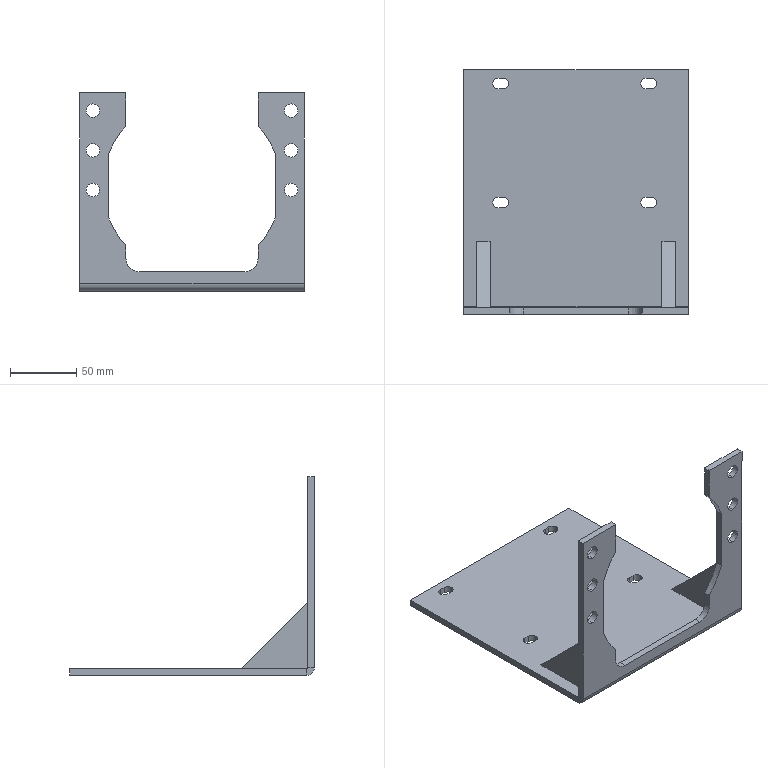Part | SolidWorks | features Gusset 2, ICE 2, 3DProfileFeature 1, Cut 1, EdgeFlange 1, Fillet 1, FlatPattern 1, HoleWzd 1, LPattern 1, MirrorPattern 1, SMBaseFlange 1, SheetMetal 1 | 3 solids | 70 faces | box 170 x 185 x 150 mm | volume 223380 mm3 | plane 38 | cylinder 32 | commonest cylinder face diameters 8 x12 10.2 x12 135 x4 20 x2 1.467 x1 11.467 x1